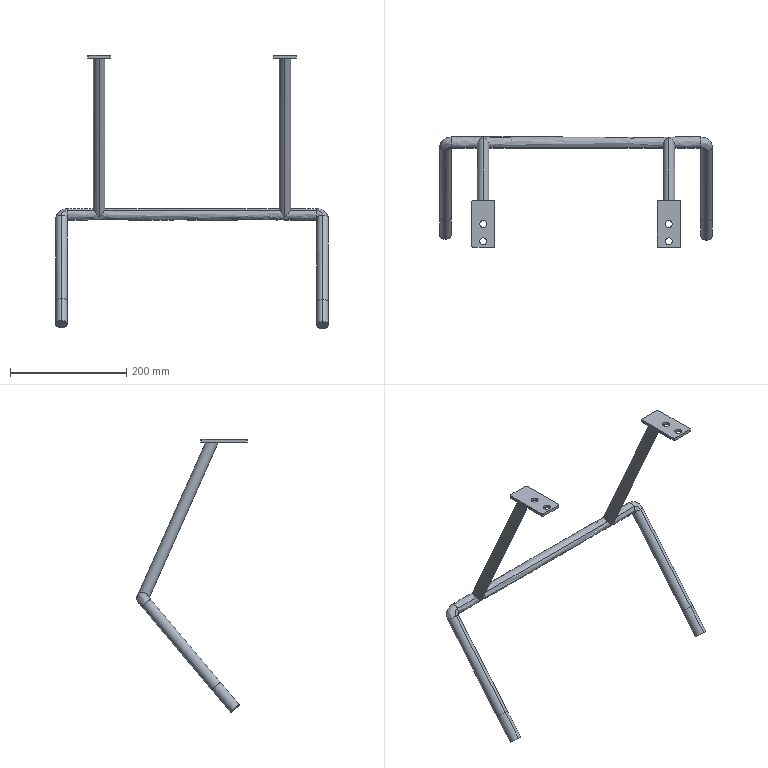Part | SolidWorks | features BaseBody 1 | 1 solid | 48 faces | box 470.221 x 190.46 x 471.381 mm | volume 503969 mm3 | cylinder 20 | plane 18 | spline 10 | commonest cylinder face diameters 12 x8 20 x8 4 x4